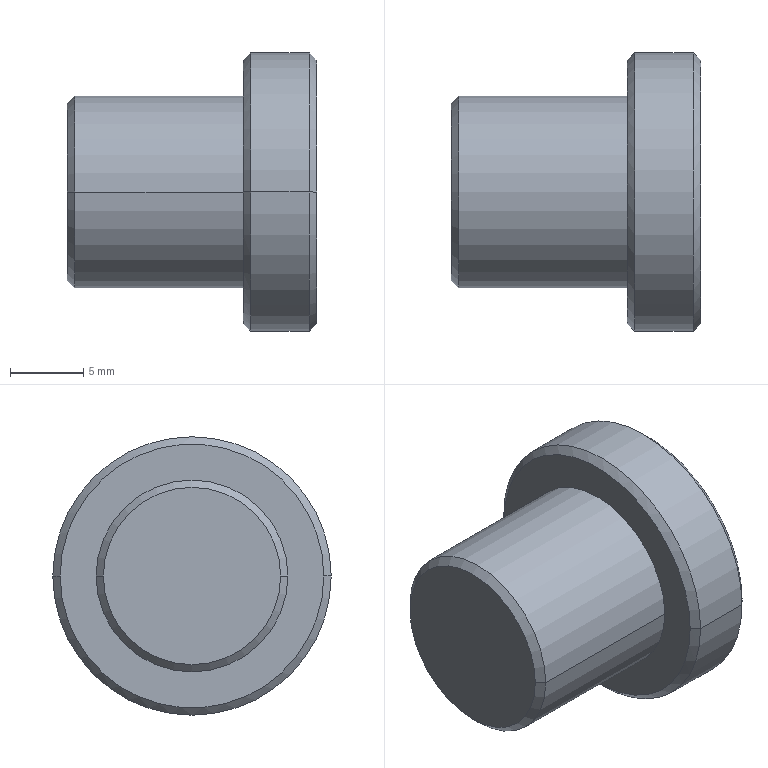Part | SolidWorks | features Chamfer 1, ICE 1, Revolution 1 | 1 solid | 20 faces | box 17 x 19 x 19 mm | volume 2888 mm3 | plane 10 | cone 6 | cylinder 4 | commonest cylinder face diameters 13.1 x2 19 x2
STEP:
#1=CARTESIAN_POINT('',(0.,-6.05,0.));
#2=VERTEX_POINT('',#1);
#3=CARTESIAN_POINT('',(0.,6.05,0.));
#4=VERTEX_POINT('',#3);
#5=CARTESIAN_POINT('',(0.,0.,0.));
#6=DIRECTION('',(-1.,0.,0.));
#7=DIRECTION('',(0.,-1.,0.));
#8=AXIS2_PLACEMENT_3D('',#5,#6,#7);
#9=CIRCLE('',#8,6.05);
#10=EDGE_CURVE('',#2,#4,#9,.T.);
#11=ORIENTED_EDGE('',*,*,#10,.F.);
#12=CARTESIAN_POINT('',(0.5,-6.55,0.));
#13=VERTEX_POINT('',#12);
#14=CARTESIAN_POINT('',(0.5,-6.55,0.));
#15=DIRECTION('',(0.7071,-0.7071,0.));
#16=VECTOR('',#15,1000.);
#17=LINE('',#14,#16);
#18=EDGE_CURVE('',#2,#13,#17,.T.);
#19=ORIENTED_EDGE('',*,*,#18,.T.);
#20=CARTESIAN_POINT('',(0.5,6.55,0.));
#21=VERTEX_POINT('',#20);
#22=CARTESIAN_POINT('',(0.5,0.,0.));
#23=DIRECTION('',(1.,0.,0.));
#24=DIRECTION('',(0.,-1.,0.));
#25=AXIS2_PLACEMENT_3D('',#22,#23,#24);
#26=CIRCLE('',#25,6.55);
#27=EDGE_CURVE('',#21,#13,#26,.T.);
#28=ORIENTED_EDGE('',*,*,#27,.F.);
#29=CARTESIAN_POINT('',(0.5,6.55,0.));
#30=DIRECTION('',(0.7071,0.7071,0.));
#31=VECTOR('',#30,1000.);
#32=LINE('',#29,#31);
#33=EDGE_CURVE('',#4,#21,#32,.T.);
#34=ORIENTED_EDGE('',*,*,#33,.F.);
#35=EDGE_LOOP('',(#11,#19,#28,#34));
#36=FACE_OUTER_BOUND('',#35,.T.);
#37=CARTESIAN_POINT('',(0.5,0.,0.));
#38=DIRECTION('',(1.,0.,0.));
#39=DIRECTION('',(0.,1.,0.));
#40=AXIS2_PLACEMENT_3D('',#37,#38,#39);
#41=CONICAL_SURFACE('',#40,6.55,0.7854);
#42=ADVANCED_FACE('',(#36),#41,.T.);
#43=CARTESIAN_POINT('',(12.,-9.,0.));
#44=VERTEX_POINT('',#43);
#45=CARTESIAN_POINT('',(12.,9.,0.));
#46=VERTEX_POINT('',#45);
#47=CARTESIAN_POINT('',(12.,0.,0.));
#48=DIRECTION('',(-1.,0.,0.));
#49=DIRECTION('',(0.,-1.,0.));
#50=AXIS2_PLACEMENT_3D('',#47,#48,#49);
#51=CIRCLE('',#50,9.);
#52=EDGE_CURVE('',#44,#46,#51,.T.);
#53=ORIENTED_EDGE('',*,*,#52,.F.);
#54=CARTESIAN_POINT('',(12.5,-9.5,0.));
#55=VERTEX_POINT('',#54);
#56=CARTESIAN_POINT('',(12.5,-9.5,0.));
#57=DIRECTION('',(0.7071,-0.7071,0.));
#58=VECTOR('',#57,1000.);
#59=LINE('',#56,#58);
#60=EDGE_CURVE('',#44,#55,#59,.T.);
#61=ORIENTED_EDGE('',*,*,#60,.T.);
#62=CARTESIAN_POINT('',(12.5,9.5,0.));
#63=VERTEX_POINT('',#62);
#64=CARTESIAN_POINT('',(12.5,0.,0.));
#65=DIRECTION('',(1.,0.,0.));
#66=DIRECTION('',(0.,-1.,0.));
#67=AXIS2_PLACEMENT_3D('',#64,#65,#66);
#68=CIRCLE('',#67,9.5);
#69=EDGE_CURVE('',#63,#55,#68,.T.);
#70=ORIENTED_EDGE('',*,*,#69,.F.);
#71=CARTESIAN_POINT('',(12.5,9.5,0.));
#72=DIRECTION('',(0.7071,0.7071,0.));
#73=VECTOR('',#72,1000.);
#74=LINE('',#71,#73);
#75=EDGE_CURVE('',#46,#63,#74,.T.);
#76=ORIENTED_EDGE('',*,*,#75,.F.);
#77=EDGE_LOOP('',(#53,#61,#70,#76));
#78=FACE_OUTER_BOUND('',#77,.T.);
#79=CARTESIAN_POINT('',(12.5,0.,0.));
#80=DIRECTION('',(1.,0.,0.));
#81=DIRECTION('',(0.,1.,0.));
#82=AXIS2_PLACEMENT_3D('',#79,#80,#81);
#83=CONICAL_SURFACE('',#82,9.5,0.7854);
#84=ADVANCED_FACE('',(#78),#83,.T.);
#85=CARTESIAN_POINT('',(17.,9.,0.));
#86=VERTEX_POINT('',#85);
#87=CARTESIAN_POINT('',(17.,-9.,0.));
#88=VERTEX_POINT('',#87);
#89=CARTESIAN_POINT('',(17.,0.,0.));
#90=DIRECTION('',(1.,0.,0.));
#91=DIRECTION('',(0.,1.,0.));
#92=AXIS2_PLACEMENT_3D('',#89,#90,#91);
#93=CIRCLE('',#92,9.);
#94=EDGE_CURVE('',#86,#88,#93,.T.);
#95=ORIENTED_EDGE('',*,*,#94,.F.);
#96=CARTESIAN_POINT('',(16.5,9.5,0.));
#97=VERTEX_POINT('',#96);
#98=CARTESIAN_POINT('',(17.,9.,0.));
#99=DIRECTION('',(-0.7071,0.7071,0.));
#100=VECTOR('',#99,1000.);
#101=LINE('',#98,#100);
#102=EDGE_CURVE('',#86,#97,#101,.T.);
#103=ORIENTED_EDGE('',*,*,#102,.T.);
#104=CARTESIAN_POINT('',(16.5,-9.5,0.));
#105=VERTEX_POINT('',#104);
#106=CARTESIAN_POINT('',(16.5,0.,0.));
#107=DIRECTION('',(-1.,0.,0.));
#108=DIRECTION('',(0.,1.,0.));
#109=AXIS2_PLACEMENT_3D('',#106,#107,#108);
#110=CIRCLE('',#109,9.5);
#111=EDGE_CURVE('',#105,#97,#110,.T.);
#112=ORIENTED_EDGE('',*,*,#111,.F.);
#113=CARTESIAN_POINT('',(17.,-9.,0.));
#114=DIRECTION('',(-0.7071,-0.7071,0.));
#115=VECTOR('',#114,1000.);
#116=LINE('',#113,#115);
#117=EDGE_CURVE('',#88,#105,#116,.T.);
#118=ORIENTED_EDGE('',*,*,#117,.F.);
#119=EDGE_LOOP('',(#95,#103,#112,#118));
#120=FACE_OUTER_BOUND('',#119,.T.);
#121=CARTESIAN_POINT('',(17.,0.,0.));
#122=DIRECTION('',(-1.,0.,0.));
#123=DIRECTION('',(0.,-1.,0.));
#124=AXIS2_PLACEMENT_3D('',#121,#122,#123);
#125=CONICAL_SURFACE('',#124,9.,0.7854);
#126=ADVANCED_FACE('',(#120),#125,.T.);
#127=ORIENTED_EDGE('',*,*,#69,.T.);
#128=CARTESIAN_POINT('',(17.,-9.5,0.));
#129=DIRECTION('',(1.,0.,0.));
#130=VECTOR('',#129,1000.);
#131=LINE('',#128,#130);
#132=EDGE_CURVE('',#55,#105,#131,.T.);
#133=ORIENTED_EDGE('',*,*,#132,.T.);
#134=ORIENTED_EDGE('',*,*,#111,.T.);
#135=CARTESIAN_POINT('',(17.,9.5,0.));
#136=DIRECTION('',(1.,0.,0.));
#137=VECTOR('',#136,1000.);
#138=LINE('',#135,#137);
#139=EDGE_CURVE('',#63,#97,#138,.T.);
#140=ORIENTED_EDGE('',*,*,#139,.F.);
#141=EDGE_LOOP('',(#127,#133,#134,#140));
#142=FACE_OUTER_BOUND('',#141,.T.);
#143=CARTESIAN_POINT('',(17.,0.,0.));
#144=DIRECTION('',(1.,0.,0.));
#145=DIRECTION('',(0.,1.,0.));
#146=AXIS2_PLACEMENT_3D('',#143,#144,#145);
#147=CYLINDRICAL_SURFACE('',#146,9.5);
#148=ADVANCED_FACE('',(#142),#147,.T.);
#149=ORIENTED_EDGE('',*,*,#27,.T.);
#150=CARTESIAN_POINT('',(12.,-6.55,0.));
#151=VERTEX_POINT('',#150);
#152=CARTESIAN_POINT('',(17.,-6.55,0.));
#153=DIRECTION('',(1.,0.,0.));
#154=VECTOR('',#153,1000.);
#155=LINE('',#152,#154);
#156=EDGE_CURVE('',#13,#151,#155,.T.);
#157=ORIENTED_EDGE('',*,*,#156,.T.);
#158=CARTESIAN_POINT('',(12.,6.55,0.));
#159=VERTEX_POINT('',#158);
#160=CARTESIAN_POINT('',(12.,0.,0.));
#161=DIRECTION('',(1.,0.,0.));
#162=DIRECTION('',(0.,1.,0.));
#163=AXIS2_PLACEMENT_3D('',#160,#161,#162);
#164=CIRCLE('',#163,6.55);
#165=EDGE_CURVE('',#159,#151,#164,.T.);
#166=ORIENTED_EDGE('',*,*,#165,.F.);
#167=CARTESIAN_POINT('',(17.,6.55,0.));
#168=DIRECTION('',(1.,0.,0.));
#169=VECTOR('',#168,1000.);
#170=LINE('',#167,#169);
#171=EDGE_CURVE('',#21,#159,#170,.T.);
#172=ORIENTED_EDGE('',*,*,#171,.F.);
#173=EDGE_LOOP('',(#149,#157,#166,#172));
#174=FACE_OUTER_BOUND('',#173,.T.);
#175=CARTESIAN_POINT('',(17.,0.,0.));
#176=DIRECTION('',(1.,0.,0.));
#177=DIRECTION('',(0.,1.,0.));
#178=AXIS2_PLACEMENT_3D('',#175,#176,#177);
#179=CYLINDRICAL_SURFACE('',#178,6.55);
#180=ADVANCED_FACE('',(#174),#179,.T.);
#181=CARTESIAN_POINT('',(0.,0.,0.));
#182=DIRECTION('',(-1.,0.,0.));
#183=DIRECTION('',(0.,-1.,0.));
#184=AXIS2_PLACEMENT_3D('',#181,#182,#183);
#185=CIRCLE('',#184,6.05);
#186=EDGE_CURVE('',#4,#2,#185,.T.);
#187=ORIENTED_EDGE('',*,*,#186,.T.);
#188=ORIENTED_EDGE('',*,*,#10,.T.);
#189=EDGE_LOOP('',(#187,#188));
#190=FACE_OUTER_BOUND('',#189,.T.);
#191=CARTESIAN_POINT('',(0.,0.,0.));
#192=DIRECTION('',(-1.,0.,0.));
#193=DIRECTION('',(0.,-1.,0.));
#194=AXIS2_PLACEMENT_3D('',#191,#192,#193);
#195=PLANE('',#194);
#196=ADVANCED_FACE('',(#190),#195,.T.);
#197=ORIENTED_EDGE('',*,*,#156,.F.);
#198=CARTESIAN_POINT('',(0.5,0.,0.));
#199=DIRECTION('',(1.,0.,0.));
#200=DIRECTION('',(0.,-1.,0.));
#201=AXIS2_PLACEMENT_3D('',#198,#199,#200);
#202=CIRCLE('',#201,6.55);
#203=EDGE_CURVE('',#13,#21,#202,.T.);
#204=ORIENTED_EDGE('',*,*,#203,.T.);
#205=ORIENTED_EDGE('',*,*,#171,.T.);
#206=CARTESIAN_POINT('',(12.,0.,0.));
#207=DIRECTION('',(1.,0.,0.));
#208=DIRECTION('',(0.,1.,0.));
#209=AXIS2_PLACEMENT_3D('',#206,#207,#208);
#210=CIRCLE('',#209,6.55);
#211=EDGE_CURVE('',#151,#159,#210,.T.);
#212=ORIENTED_EDGE('',*,*,#211,.F.);
#213=EDGE_LOOP('',(#197,#204,#205,#212));
#214=FACE_OUTER_BOUND('',#213,.T.);
#215=CARTESIAN_POINT('',(17.,0.,0.));
#216=DIRECTION('',(1.,0.,0.));
#217=DIRECTION('',(0.,1.,0.));
#218=AXIS2_PLACEMENT_3D('',#215,#216,#217);
#219=CYLINDRICAL_SURFACE('',#218,6.55);
#220=ADVANCED_FACE('',(#214),#219,.T.);
#221=CARTESIAN_POINT('',(12.,0.,0.));
#222=DIRECTION('',(-1.,0.,0.));
#223=DIRECTION('',(0.,-1.,0.));
#224=AXIS2_PLACEMENT_3D('',#221,#222,#223);
#225=CIRCLE('',#224,9.);
#226=EDGE_CURVE('',#46,#44,#225,.T.);
#227=ORIENTED_EDGE('',*,*,#226,.T.);
#228=ORIENTED_EDGE('',*,*,#52,.T.);
#229=EDGE_LOOP('',(#227,#228));
#230=FACE_OUTER_BOUND('',#229,.T.);
#231=ORIENTED_EDGE('',*,*,#165,.T.);
#232=ORIENTED_EDGE('',*,*,#211,.T.);
#233=EDGE_LOOP('',(#231,#232));
#234=FACE_BOUND('',#233,.T.);
#235=CARTESIAN_POINT('',(12.,6.55,0.));
#236=DIRECTION('',(-1.,0.,0.));
#237=DIRECTION('',(0.,-1.,0.));
#238=AXIS2_PLACEMENT_3D('',#235,#236,#237);
#239=PLANE('',#238);
#240=ADVANCED_FACE('',(#230,#234),#239,.T.);
#241=ORIENTED_EDGE('',*,*,#132,.F.);
#242=CARTESIAN_POINT('',(12.5,0.,0.));
#243=DIRECTION('',(1.,0.,0.));
#244=DIRECTION('',(0.,-1.,0.));
#245=AXIS2_PLACEMENT_3D('',#242,#243,#244);
#246=CIRCLE('',#245,9.5);
#247=EDGE_CURVE('',#55,#63,#246,.T.);
#248=ORIENTED_EDGE('',*,*,#247,.T.);
#249=ORIENTED_EDGE('',*,*,#139,.T.);
#250=CARTESIAN_POINT('',(16.5,0.,0.));
#251=DIRECTION('',(-1.,0.,0.));
#252=DIRECTION('',(0.,1.,0.));
#253=AXIS2_PLACEMENT_3D('',#250,#251,#252);
#254=CIRCLE('',#253,9.5);
#255=EDGE_CURVE('',#97,#105,#254,.T.);
#256=ORIENTED_EDGE('',*,*,#255,.T.);
#257=EDGE_LOOP('',(#241,#248,#249,#256));
#258=FACE_OUTER_BOUND('',#257,.T.);
#259=CARTESIAN_POINT('',(17.,0.,0.));
#260=DIRECTION('',(1.,0.,0.));
#261=DIRECTION('',(0.,1.,0.));
#262=AXIS2_PLACEMENT_3D('',#259,#260,#261);
#263=CYLINDRICAL_SURFACE('',#262,9.5);
#264=ADVANCED_FACE('',(#258),#263,.T.);
#265=CARTESIAN_POINT('',(17.,0.,0.));
#266=DIRECTION('',(1.,0.,0.));
#267=DIRECTION('',(0.,1.,0.));
#268=AXIS2_PLACEMENT_3D('',#265,#266,#267);
#269=CIRCLE('',#268,9.);
#270=EDGE_CURVE('',#88,#86,#269,.T.);
#271=ORIENTED_EDGE('',*,*,#270,.T.);
#272=ORIENTED_EDGE('',*,*,#94,.T.);
#273=EDGE_LOOP('',(#271,#272));
#274=FACE_OUTER_BOUND('',#273,.T.);
#275=CARTESIAN_POINT('',(17.,2.021,-3.5));
#276=VERTEX_POINT('',#275);
#277=CARTESIAN_POINT('',(17.,4.041,0.));
#278=VERTEX_POINT('',#277);
#279=CARTESIAN_POINT('',(17.,2.021,-3.5));
#280=DIRECTION('',(0.,0.5,0.866));
#281=VECTOR('',#280,1000.);
#282=LINE('',#279,#281);
#283=EDGE_CURVE('',#276,#278,#282,.T.);
#284=ORIENTED_EDGE('',*,*,#283,.F.);
#285=CARTESIAN_POINT('',(17.,-2.021,-3.5));
#286=VERTEX_POINT('',#285);
#287=CARTESIAN_POINT('',(17.,-2.021,-3.5));
#288=DIRECTION('',(0.,1.,0.));
#289=VECTOR('',#288,1000.);
#290=LINE('',#287,#289);
#291=EDGE_CURVE('',#286,#276,#290,.T.);
#292=ORIENTED_EDGE('',*,*,#291,.F.);
#293=CARTESIAN_POINT('',(17.,-4.041,0.));
#294=VERTEX_POINT('',#293);
#295=CARTESIAN_POINT('',(17.,-4.041,0.));
#296=DIRECTION('',(0.,0.5,-0.866));
#297=VECTOR('',#296,1000.);
#298=LINE('',#295,#297);
#299=EDGE_CURVE('',#294,#286,#298,.T.);
#300=ORIENTED_EDGE('',*,*,#299,.F.);
#301=CARTESIAN_POINT('',(17.,-2.021,3.5));
#302=VERTEX_POINT('',#301);
#303=CARTESIAN_POINT('',(17.,-2.021,3.5));
#304=DIRECTION('',(0.,-0.5,-0.866));
#305=VECTOR('',#304,1000.);
#306=LINE('',#303,#305);
#307=EDGE_CURVE('',#302,#294,#306,.T.);
#308=ORIENTED_EDGE('',*,*,#307,.F.);
#309=CARTESIAN_POINT('',(17.,2.021,3.5));
#310=VERTEX_POINT('',#309);
#311=CARTESIAN_POINT('',(17.,2.021,3.5));
#312=DIRECTION('',(0.,-1.,0.));
#313=VECTOR('',#312,1000.);
#314=LINE('',#311,#313);
#315=EDGE_CURVE('',#310,#302,#314,.T.);
#316=ORIENTED_EDGE('',*,*,#315,.F.);
#317=CARTESIAN_POINT('',(17.,4.041,0.));
#318=DIRECTION('',(0.,-0.5,0.866));
#319=VECTOR('',#318,1000.);
#320=LINE('',#317,#319);
#321=EDGE_CURVE('',#278,#310,#320,.T.);
#322=ORIENTED_EDGE('',*,*,#321,.F.);
#323=EDGE_LOOP('',(#284,#292,#300,#308,#316,#322));
#324=FACE_BOUND('',#323,.T.);
#325=CARTESIAN_POINT('',(17.,9.5,0.));
#326=DIRECTION('',(1.,0.,0.));
#327=DIRECTION('',(0.,1.,0.));
#328=AXIS2_PLACEMENT_3D('',#325,#326,#327);
#329=PLANE('',#328);
#330=ADVANCED_FACE('',(#274,#324),#329,.T.);
#331=ORIENTED_EDGE('',*,*,#283,.T.);
#332=CARTESIAN_POINT('',(14.,4.041,0.));
#333=VERTEX_POINT('',#332);
#334=CARTESIAN_POINT('',(14.,4.041,0.));
#335=DIRECTION('',(1.,0.,0.));
#336=VECTOR('',#335,1000.);
#337=LINE('',#334,#336);
#338=EDGE_CURVE('',#333,#278,#337,.T.);
#339=ORIENTED_EDGE('',*,*,#338,.F.);
#340=CARTESIAN_POINT('',(14.,2.021,-3.5));
#341=VERTEX_POINT('',#340);
#342=CARTESIAN_POINT('',(14.,2.021,-3.5));
#343=DIRECTION('',(0.,0.5,0.866));
#344=VECTOR('',#343,1000.);
#345=LINE('',#342,#344);
#346=EDGE_CURVE('',#341,#333,#345,.T.);
#347=ORIENTED_EDGE('',*,*,#346,.F.);
#348=CARTESIAN_POINT('',(14.,2.021,-3.5));
#349=DIRECTION('',(1.,0.,0.));
#350=VECTOR('',#349,1000.);
#351=LINE('',#348,#350);
#352=EDGE_CURVE('',#341,#276,#351,.T.);
#353=ORIENTED_EDGE('',*,*,#352,.T.);
#354=EDGE_LOOP('',(#331,#339,#347,#353));
#355=FACE_OUTER_BOUND('',#354,.T.);
#356=CARTESIAN_POINT('',(14.,2.021,-3.5));
#357=DIRECTION('',(0.,0.866,-0.5));
#358=DIRECTION('',(0.,0.5,0.866));
#359=AXIS2_PLACEMENT_3D('',#356,#357,#358);
#360=PLANE('',#359);
#361=ADVANCED_FACE('',(#355),#360,.F.);
#362=ORIENTED_EDGE('',*,*,#291,.T.);
#363=ORIENTED_EDGE('',*,*,#352,.F.);
#364=CARTESIAN_POINT('',(14.,-2.021,-3.5));
#365=VERTEX_POINT('',#364);
#366=CARTESIAN_POINT('',(14.,-2.021,-3.5));
#367=DIRECTION('',(0.,1.,0.));
#368=VECTOR('',#367,1000.);
#369=LINE('',#366,#368);
#370=EDGE_CURVE('',#365,#341,#369,.T.);
#371=ORIENTED_EDGE('',*,*,#370,.F.);
#372=CARTESIAN_POINT('',(14.,-2.021,-3.5));
#373=DIRECTION('',(1.,0.,0.));
#374=VECTOR('',#373,1000.);
#375=LINE('',#372,#374);
#376=EDGE_CURVE('',#365,#286,#375,.T.);
#377=ORIENTED_EDGE('',*,*,#376,.T.);
#378=EDGE_LOOP('',(#362,#363,#371,#377));
#379=FACE_OUTER_BOUND('',#378,.T.);
#380=CARTESIAN_POINT('',(14.,-2.021,-3.5));
#381=DIRECTION('',(0.,0.,-1.));
#382=DIRECTION('',(0.,1.,0.));
#383=AXIS2_PLACEMENT_3D('',#380,#381,#382);
#384=PLANE('',#383);
#385=ADVANCED_FACE('',(#379),#384,.F.);
#386=ORIENTED_EDGE('',*,*,#299,.T.);
#387=ORIENTED_EDGE('',*,*,#376,.F.);
#388=CARTESIAN_POINT('',(14.,-4.041,0.));
#389=VERTEX_POINT('',#388);
#390=CARTESIAN_POINT('',(14.,-4.041,0.));
#391=DIRECTION('',(0.,0.5,-0.866));
#392=VECTOR('',#391,1000.);
#393=LINE('',#390,#392);
#394=EDGE_CURVE('',#389,#365,#393,.T.);
#395=ORIENTED_EDGE('',*,*,#394,.F.);
#396=CARTESIAN_POINT('',(14.,-4.041,0.));
#397=DIRECTION('',(1.,0.,0.));
#398=VECTOR('',#397,1000.);
#399=LINE('',#396,#398);
#400=EDGE_CURVE('',#389,#294,#399,.T.);
#401=ORIENTED_EDGE('',*,*,#400,.T.);
#402=EDGE_LOOP('',(#386,#387,#395,#401));
#403=FACE_OUTER_BOUND('',#402,.T.);
#404=CARTESIAN_POINT('',(14.,-4.041,0.));
#405=DIRECTION('',(0.,-0.866,-0.5));
#406=DIRECTION('',(0.,0.5,-0.866));
#407=AXIS2_PLACEMENT_3D('',#404,#405,#406);
#408=PLANE('',#407);
#409=ADVANCED_FACE('',(#403),#408,.F.);
#410=ORIENTED_EDGE('',*,*,#307,.T.);
#411=ORIENTED_EDGE('',*,*,#400,.F.);
#412=CARTESIAN_POINT('',(14.,-2.021,3.5));
#413=VERTEX_POINT('',#412);
#414=CARTESIAN_POINT('',(14.,-2.021,3.5));
#415=DIRECTION('',(0.,-0.5,-0.866));
#416=VECTOR('',#415,1000.);
#417=LINE('',#414,#416);
#418=EDGE_CURVE('',#413,#389,#417,.T.);
#419=ORIENTED_EDGE('',*,*,#418,.F.);
#420=CARTESIAN_POINT('',(14.,-2.021,3.5));
#421=DIRECTION('',(1.,0.,0.));
#422=VECTOR('',#421,1000.);
#423=LINE('',#420,#422);
#424=EDGE_CURVE('',#413,#302,#423,.T.);
#425=ORIENTED_EDGE('',*,*,#424,.T.);
#426=EDGE_LOOP('',(#410,#411,#419,#425));
#427=FACE_OUTER_BOUND('',#426,.T.);
#428=CARTESIAN_POINT('',(14.,-2.021,3.5));
#429=DIRECTION('',(0.,-0.866,0.5));
#430=DIRECTION('',(0.,-0.5,-0.866));
#431=AXIS2_PLACEMENT_3D('',#428,#429,#430);
#432=PLANE('',#431);
#433=ADVANCED_FACE('',(#427),#432,.F.);
#434=ORIENTED_EDGE('',*,*,#315,.T.);
#435=ORIENTED_EDGE('',*,*,#424,.F.);
#436=CARTESIAN_POINT('',(14.,2.021,3.5));
#437=VERTEX_POINT('',#436);
#438=CARTESIAN_POINT('',(14.,2.021,3.5));
#439=DIRECTION('',(0.,-1.,0.));
#440=VECTOR('',#439,1000.);
#441=LINE('',#438,#440);
#442=EDGE_CURVE('',#437,#413,#441,.T.);
#443=ORIENTED_EDGE('',*,*,#442,.F.);
#444=CARTESIAN_POINT('',(14.,2.021,3.5));
#445=DIRECTION('',(1.,0.,0.));
#446=VECTOR('',#445,1000.);
#447=LINE('',#444,#446);
#448=EDGE_CURVE('',#437,#310,#447,.T.);
#449=ORIENTED_EDGE('',*,*,#448,.T.);
#450=EDGE_LOOP('',(#434,#435,#443,#449));
#451=FACE_OUTER_BOUND('',#450,.T.);
#452=CARTESIAN_POINT('',(14.,2.021,3.5));
#453=DIRECTION('',(0.,0.,1.));
#454=DIRECTION('',(1.,0.,0.));
#455=AXIS2_PLACEMENT_3D('',#452,#453,#454);
#456=PLANE('',#455);
#457=ADVANCED_FACE('',(#451),#456,.F.);
#458=ORIENTED_EDGE('',*,*,#321,.T.);
#459=ORIENTED_EDGE('',*,*,#448,.F.);
#460=CARTESIAN_POINT('',(14.,4.041,0.));
#461=DIRECTION('',(0.,-0.5,0.866));
#462=VECTOR('',#461,1000.);
#463=LINE('',#460,#462);
#464=EDGE_CURVE('',#333,#437,#463,.T.);
#465=ORIENTED_EDGE('',*,*,#464,.F.);
#466=ORIENTED_EDGE('',*,*,#338,.T.);
#467=EDGE_LOOP('',(#458,#459,#465,#466));
#468=FACE_OUTER_BOUND('',#467,.T.);
#469=CARTESIAN_POINT('',(14.,4.041,0.));
#470=DIRECTION('',(0.,0.866,0.5));
#471=DIRECTION('',(0.,-0.5,0.866));
#472=AXIS2_PLACEMENT_3D('',#469,#470,#471);
#473=PLANE('',#472);
#474=ADVANCED_FACE('',(#468),#473,.F.);
#475=ORIENTED_EDGE('',*,*,#346,.T.);
#476=ORIENTED_EDGE('',*,*,#464,.T.);
#477=ORIENTED_EDGE('',*,*,#442,.T.);
#478=ORIENTED_EDGE('',*,*,#418,.T.);
#479=ORIENTED_EDGE('',*,*,#394,.T.);
#480=ORIENTED_EDGE('',*,*,#370,.T.);
#481=EDGE_LOOP('',(#475,#476,#477,#478,#479,#480));
#482=FACE_OUTER_BOUND('',#481,.T.);
#483=CARTESIAN_POINT('',(14.,0.,0.));
#484=DIRECTION('',(1.,0.,0.));
#485=DIRECTION('',(0.,0.,-1.));
#486=AXIS2_PLACEMENT_3D('',#483,#484,#485);
#487=PLANE('',#486);
#488=ADVANCED_FACE('',(#482),#487,.T.);
#489=ORIENTED_EDGE('',*,*,#102,.F.);
#490=ORIENTED_EDGE('',*,*,#270,.F.);
#491=ORIENTED_EDGE('',*,*,#117,.T.);
#492=ORIENTED_EDGE('',*,*,#255,.F.);
#493=EDGE_LOOP('',(#489,#490,#491,#492));
#494=FACE_OUTER_BOUND('',#493,.T.);
#495=CARTESIAN_POINT('',(17.,0.,0.));
#496=DIRECTION('',(-1.,0.,0.));
#497=DIRECTION('',(0.,-1.,0.));
#498=AXIS2_PLACEMENT_3D('',#495,#496,#497);
#499=CONICAL_SURFACE('',#498,9.,0.7854);
#500=ADVANCED_FACE('',(#494),#499,.T.);
#501=ORIENTED_EDGE('',*,*,#60,.F.);
#502=ORIENTED_EDGE('',*,*,#226,.F.);
#503=ORIENTED_EDGE('',*,*,#75,.T.);
#504=ORIENTED_EDGE('',*,*,#247,.F.);
#505=EDGE_LOOP('',(#501,#502,#503,#504));
#506=FACE_OUTER_BOUND('',#505,.T.);
#507=CARTESIAN_POINT('',(12.5,0.,0.));
#508=DIRECTION('',(1.,0.,0.));
#509=DIRECTION('',(0.,1.,0.));
#510=AXIS2_PLACEMENT_3D('',#507,#508,#509);
#511=CONICAL_SURFACE('',#510,9.5,0.7854);
#512=ADVANCED_FACE('',(#506),#511,.T.);
#513=ORIENTED_EDGE('',*,*,#18,.F.);
#514=ORIENTED_EDGE('',*,*,#186,.F.);
#515=ORIENTED_EDGE('',*,*,#33,.T.);
#516=ORIENTED_EDGE('',*,*,#203,.F.);
#517=EDGE_LOOP('',(#513,#514,#515,#516));
#518=FACE_OUTER_BOUND('',#517,.T.);
#519=CARTESIAN_POINT('',(0.5,0.,0.));
#520=DIRECTION('',(1.,0.,0.));
#521=DIRECTION('',(0.,1.,0.));
#522=AXIS2_PLACEMENT_3D('',#519,#520,#521);
#523=CONICAL_SURFACE('',#522,6.55,0.7854);
#524=ADVANCED_FACE('',(#518),#523,.T.);
#525=CLOSED_SHELL('',(#42,#84,#126,#148,#180,#196,#220,#240,#264,#330,#361,#385,#409,#433,#457,#474,#488,#500,#512,#524));
#526=MANIFOLD_SOLID_BREP('',#525);
#527=CARTESIAN_POINT('',(0.,0.,0.));
#528=DIRECTION('',(0.,0.,1.));
#529=DIRECTION('',(1.,0.,0.));
#530=AXIS2_PLACEMENT_3D('',#527,#528,#529);
#531=(LENGTH_UNIT()NAMED_UNIT(*)SI_UNIT(.MILLI.,.METRE.));
#532=UNCERTAINTY_MEASURE_WITH_UNIT(LENGTH_MEASURE(0.00001),#531,'','');
#533=(NAMED_UNIT(*)PLANE_ANGLE_UNIT()SI_UNIT($,.RADIAN.));
#534=(NAMED_UNIT(*)SI_UNIT($,.STERADIAN.)SOLID_ANGLE_UNIT());
#535=(GEOMETRIC_REPRESENTATION_CONTEXT(3)GLOBAL_UNCERTAINTY_ASSIGNED_CONTEXT((#532))GLOBAL_UNIT_ASSIGNED_CONTEXT((#531,#533,#534))REPRESENTATION_CONTEXT('',''));
#536=ADVANCED_BREP_SHAPE_REPRESENTATION('',(#526,#530),#535);